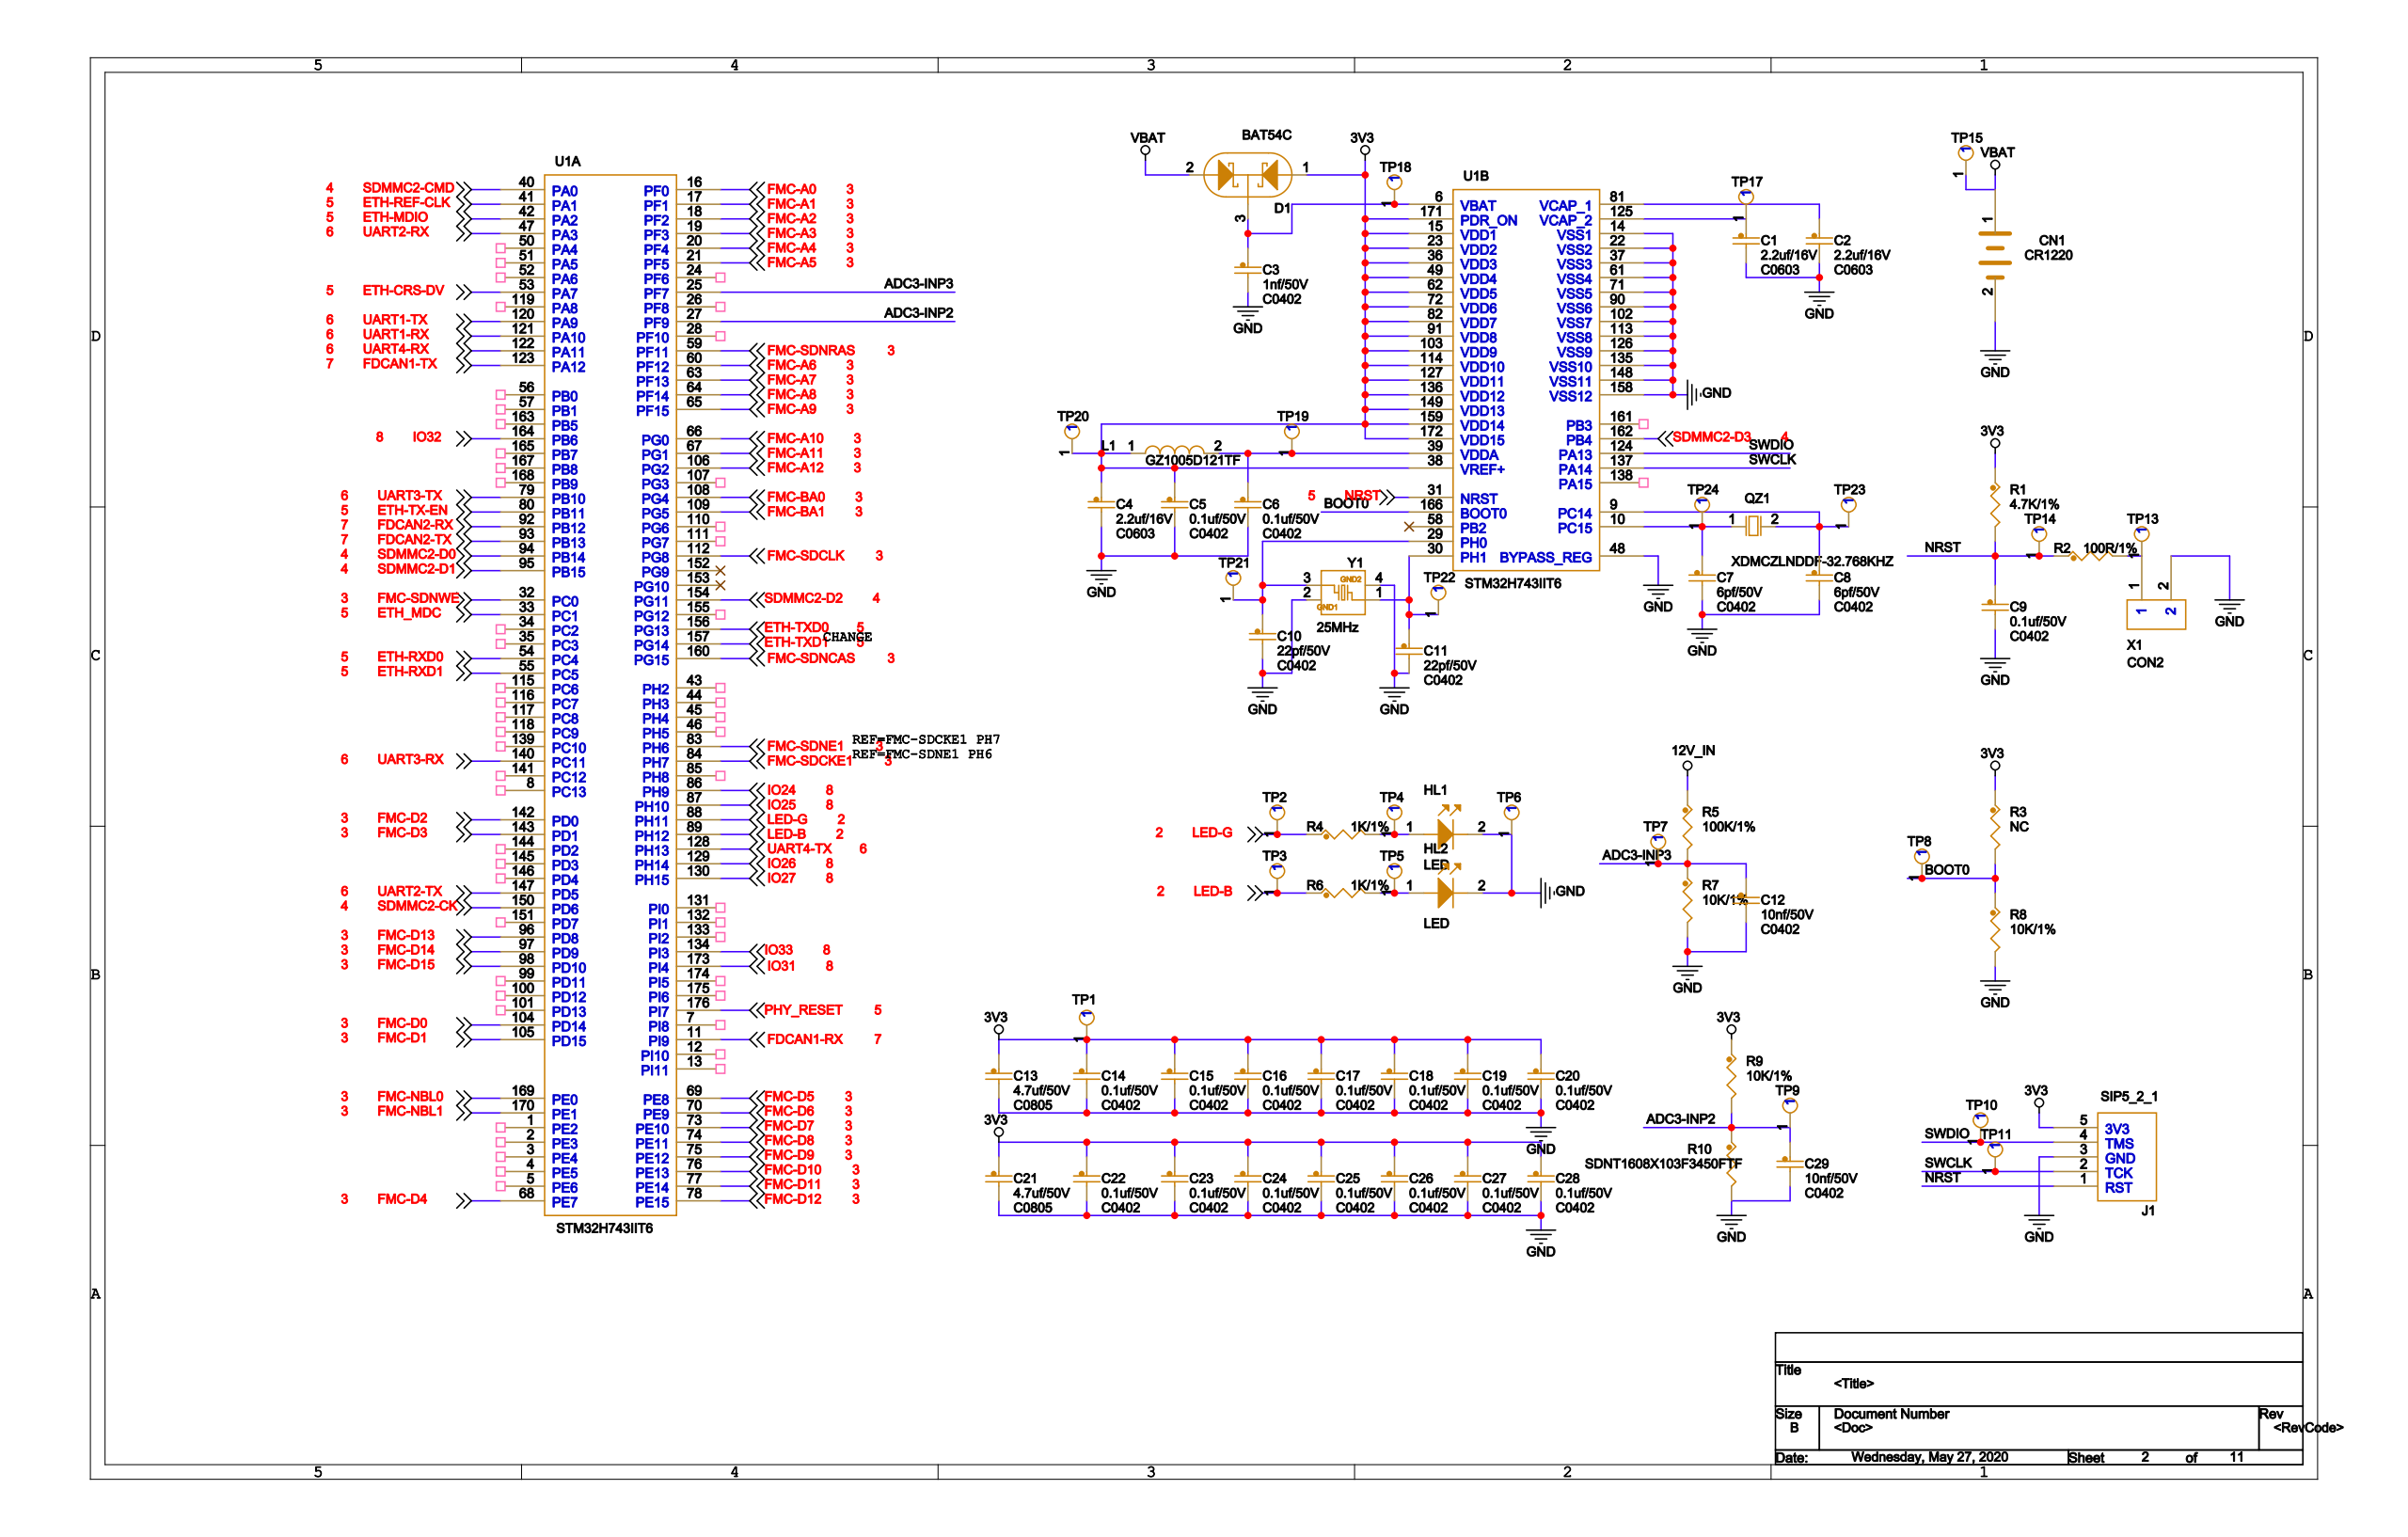Circuit board | Cadence Allegro | 521 parts | 239 nets | one sheet of the schematic
Parts on this sheet (reference | value | footprint):
C1 | 2.2uf/16V | C0603
C2 | 2.2uf/16V | C0603
C3 | 1nf/50V | C0402
C4 | 2.2uf/16V | C0603
C5 | 0.1uf/50V | C0402
C6 | 0.1uf/50V | C0402
C7 | 6pf/50V | C0402
C8 | 6pf/50V | C0402
C9 | 0.1uf/50V | C0402
C10 | 22pf/50V | C0402
C11 | 22pf/50V | C0402
C12 | 10nf/50V | C0402
C13 | 4.7uf/50V | C0805
C14 | 0.1uf/50V | C0402
C15 | 0.1uf/50V | C0402
C16 | 0.1uf/50V | C0402
C17 | 0.1uf/50V | C0402
C18 | 0.1uf/50V | C0402
C19 | 0.1uf/50V | C0402
C20 | 0.1uf/50V | C0402
C21 | 4.7uf/50V | C0805
C22 | 0.1uf/50V | C0402
C23 | 0.1uf/50V | C0402
C24 | 0.1uf/50V | C0402
C25 | 0.1uf/50V | C0402
C26 | 0.1uf/50V | C0402
C27 | 0.1uf/50V | C0402
C28 | 0.1uf/50V | C0402
C29 | 10nf/50V | C0402
CN1 | CR1220 | CR1220
D1 | BAT54C | SOT23
HL1 | LED | LED0603
HL2 | LED | LED0603
J1 | SIP5_2_1 | SIP5
L1 | GZ1005D121TF | 0402
QZ1 | XDMCZLNDDF-32.768KHZ | XTAL_SMD_3215
R1 | 4.7K/1% | 0402
R2 | 100R/1% | 0603
R3 | NC | 0402
R4 | 1K/1% | 0603
R5 | 100K/1% | 0603
R6 | 1K/1% | 0603
R7 | 10K/1% | 0402
R8 | 10K/1% | 0402
R9 | 10K/1% | 0402
R10 | SDNT1608X103F3450FTF | 0603
TP1 | TESTPOINT | TESTPOINT-33MIL
TP2 | TESTPOINT | TESTPOINT-33MIL
TP3 | TESTPOINT | TESTPOINT-33MIL
TP4 | TESTPOINT | TESTPOINT-33MIL
TP5 | TESTPOINT | TESTPOINT-33MIL
TP6 | TESTPOINT | TESTPOINT-33MIL
TP7 | TESTPOINT | TESTPOINT-33MIL
TP8 | TESTPOINT | TESTPOINT-33MIL
TP9 | TESTPOINT | TESTPOINT-33MIL
TP10 | TESTPOINT | TESTPOINT-33MIL
TP11 | TESTPOINT | TESTPOINT-33MIL
TP13 | TESTPOINT | TESTPOINT-33MIL
TP14 | TESTPOINT | TESTPOINT-33MIL
TP15 | TESTPOINT | TESTPOINT-33MIL
TP17 | TESTPOINT | TESTPOINT-33MIL
TP18 | TESTPOINT | TESTPOINT-33MIL
TP19 | TESTPOINT | TESTPOINT-33MIL
TP20 | TESTPOINT | TESTPOINT-33MIL
TP21 | TESTPOINT | TESTPOINT-33MIL
TP22 | TESTPOINT | TESTPOINT-33MIL
TP23 | TESTPOINT | TESTPOINT-33MIL
TP24 | TESTPOINT | TESTPOINT-33MIL
U1 | STM32H743IIT6 | LQFP176
X1 | CON2 | SIP2
Y1 | 25MHz | OSC_SMD3L2X2L5
Nets of these parts (net: part-pin ...):
GND: C1-2 C2-2 C3-2 C4-2 C5-2 C6-2 C7-2 C8-2 C9-2 C10-2 C11-2 C12-2 C13-2 C14-2 C15-2 C16-2 C17-2 C18-2 C19-2 C20-2 C21-2 C22-2 C23-2 C24-2 C25-2 C26-2 C27-2 C28-2 C29-2 CN1-2 HL1-2 HL2-2 J1-3 R7-2 R8-2 R10-2 TP6-1 X1-2 Y1-2 Y1-4 U1-14 U1-22 U1-37 U1-48 U1-61 U1-71 U1-90 U1-102 U1-113 U1-126 U1-135 U1-148 U1-158
12V_IN: R5-1
3V3: C4-1 C5-1 C13-1 C14-1 C15-1 C16-1 C17-1 C18-1 C19-1 C20-1 C21-1 C22-1 C23-1 C24-1 C25-1 C26-1 C27-1 C28-1 D1-1 J1-5 L1-1 R1-1 R3-1 R9-1 TP1-1 TP20-1 U1-15 U1-23 U1-36 U1-38 U1-49 U1-62 U1-72 U1-82 U1-91 U1-103 U1-114 U1-127 U1-136 U1-149 U1-159 U1-171 U1-172
SWDIO: J1-4 TP10-1 U1-124
UART3-RX: U1-140
UART3-TX: U1-79
SWCLK: J1-2 TP11-1 U1-137
UART4-RX: U1-122
UART4-TX: U1-128
N04941: R2-2 TP13-1 X1-1
NRST: C9-1 J1-1 R1-2 R2-1 TP14-1 U1-31
FDCAN2-TX: U1-93
FDCAN2-RX: U1-92
VBAT: CN1-1 D1-2 TP15-1
N05702: C1-1 TP17-1 U1-125
IO24: U1-86
IO25: U1-87
IO26: U1-129
IO27: U1-130
IO33: U1-134
N01856: C3-1 D1-3 TP18-1 U1-6
N02795: C6-1 L1-2 TP19-1 U1-39
LED-G: R4-1 TP2-1 U1-88
N04020: C10-1 TP21-1 Y1-3 U1-29
N04068: C11-1 TP22-1 Y1-1 U1-30
N06443: C8-1 QZ1-2 TP23-1 U1-9
N06439: C7-1 QZ1-1 TP24-1 U1-10
SDMMC2-D2: U1-154
SDMMC2-D3: U1-162
SDMMC2-CMD: U1-40
SDMMC2-CK: U1-150
SDMMC2-D0: U1-94
LED-B: R6-1 TP3-1 U1-89
SDMMC2-D1: U1-95
N7355274: HL1-1 R4-2 TP4-1
PHY_RESET: U1-176
ETH-TX-EN: U1-80
ETH-TXD0: U1-156
ETH-TXD1: U1-157
ETH-RXD1: U1-55
ETH-RXD0: U1-54
ETH-CRS-DV: U1-53
ETH-REF-CLK: U1-41
N7355359: HL2-1 R6-2 TP5-1
ETH_MDC: U1-33
ETH-MDIO: U1-42
ADC3-INP3: C12-1 R5-2 R7-1 TP7-1 U1-25
BOOT0: R3-2 R8-1 TP8-1 U1-166
ADC3-INP2: C29-1 R9-2 R10-1 TP9-1 U1-27
FDCAN1-RX: U1-11
UART1-TX: U1-120
UART1-RX: U1-121
FDCAN1-TX: U1-123
N05695: C2-1 U1-81
IO32: U1-164
IO31: U1-173
UART2-RX: U1-47
UART2-TX: U1-147
FMC-SDNE1: U1-83
FMC-SDNWE: U1-32
FMC-D2: U1-142
FMC-D3: U1-143
FMC-D15: U1-98
FMC-D0: U1-104
FMC-D1: U1-105
FMC-D13: U1-96
FMC-D14: U1-97
FMC-NBL0: U1-169
FMC-NBL1: U1-170
FMC-D7: U1-73
FMC-D8: U1-74
FMC-D9: U1-75
FMC-D10: U1-76
FMC-D11: U1-77
FMC-D12: U1-78
FMC-D4: U1-68
FMC-D5: U1-69
FMC-D6: U1-70
FMC-A0: U1-16
FMC-A1: U1-17
FMC-SDNRAS: U1-59
FMC-A6: U1-60
FMC-A7: U1-63
FMC-A8: U1-64
FMC-A9: U1-65
FMC-A2: U1-18
FMC-A3: U1-19
FMC-A4: U1-20
FMC-A5: U1-21
FMC-A10: U1-66
FMC-A11: U1-67
FMC-SDNCAS: U1-160
FMC-A12: U1-106
FMC-BA0: U1-108
FMC-BA1: U1-109
FMC-SDCLK: U1-112
FMC-SDCKE1: U1-84